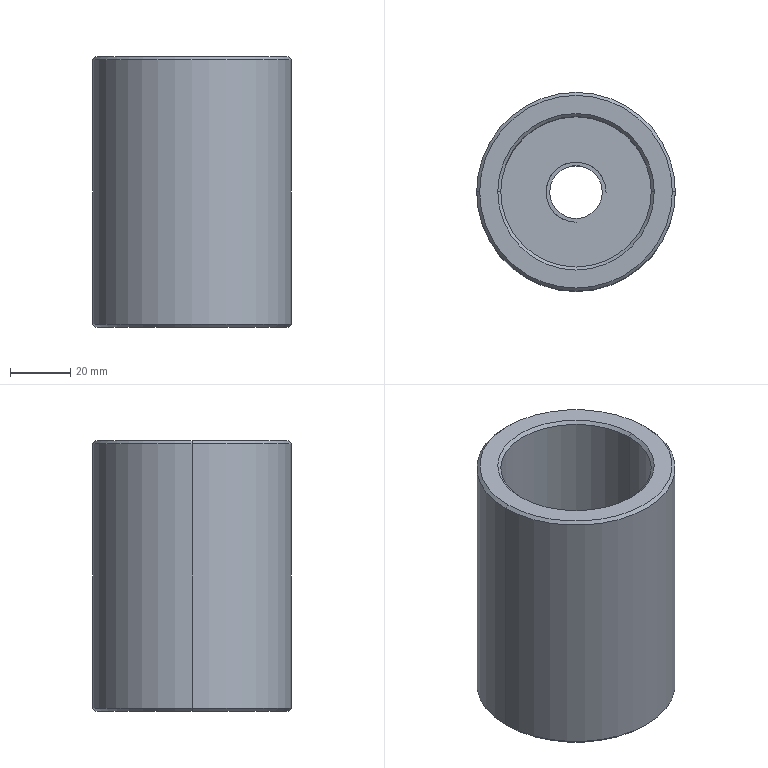Part | Creo | 1 solid | 19 faces | box 66 x 66 x 90 mm | volume 161896 mm3 | cylinder 8 | cone 6 | plane 5 | commonest cylinder face diameters 17.5 x2 50 x2 66 x2 19.94 x1 20 x1
STEP:
#1=CARTESIAN_POINT('',(-258.,289.995,-348.));
#2=VERTEX_POINT('',#1);
#3=CARTESIAN_POINT('',(-208.,289.995,-348.));
#4=VERTEX_POINT('',#3);
#5=CARTESIAN_POINT('',(-233.,289.995,-348.));
#6=DIRECTION('',(0.,0.,1.));
#7=DIRECTION('',(-1.,0.,0.));
#8=AXIS2_PLACEMENT_3D('',#5,#6,#7);
#9=CIRCLE('',#8,25.);
#10=EDGE_CURVE('',#2,#4,#9,.T.);
#11=ORIENTED_EDGE('',*,*,#10,.F.);
#12=CARTESIAN_POINT('',(-233.,289.995,-348.));
#13=DIRECTION('',(0.,0.,1.));
#14=DIRECTION('',(1.,0.,0.));
#15=AXIS2_PLACEMENT_3D('',#12,#13,#14);
#16=CIRCLE('',#15,25.);
#17=EDGE_CURVE('',#4,#2,#16,.T.);
#18=ORIENTED_EDGE('',*,*,#17,.F.);
#19=EDGE_LOOP('',(#11,#18));
#20=FACE_OUTER_BOUND('',#19,.F.);
#21=CARTESIAN_POINT('',(-241.75,289.995,-348.));
#22=VERTEX_POINT('',#21);
#23=CARTESIAN_POINT('',(-224.25,289.995,-348.));
#24=VERTEX_POINT('',#23);
#25=CARTESIAN_POINT('',(-233.,289.995,-348.));
#26=DIRECTION('',(0.,0.,-1.));
#27=DIRECTION('',(-1.,0.,0.));
#28=AXIS2_PLACEMENT_3D('',#25,#26,#27);
#29=CIRCLE('',#28,8.75);
#30=EDGE_CURVE('',#22,#24,#29,.T.);
#31=ORIENTED_EDGE('',*,*,#30,.F.);
#32=CARTESIAN_POINT('',(-233.,289.995,-348.));
#33=DIRECTION('',(0.,0.,-1.));
#34=DIRECTION('',(1.,0.,0.));
#35=AXIS2_PLACEMENT_3D('',#32,#33,#34);
#36=CIRCLE('',#35,8.75);
#37=EDGE_CURVE('',#24,#22,#36,.T.);
#38=ORIENTED_EDGE('',*,*,#37,.F.);
#39=EDGE_LOOP('',(#31,#38));
#40=FACE_BOUND('',#39,.F.);
#41=CARTESIAN_POINT('',(-233.,280.025,-348.));
#42=VERTEX_POINT('',#41);
#43=CARTESIAN_POINT('',(-233.,279.995,-348.));
#44=VERTEX_POINT('',#43);
#45=CARTESIAN_POINT('',(-233.,280.025,-348.));
#46=DIRECTION('',(0.,-1.,0.));
#47=VECTOR('',#46,0.03);
#48=LINE('',#45,#47);
#49=EDGE_CURVE('',#42,#44,#48,.T.);
#50=ORIENTED_EDGE('',*,*,#49,.F.);
#51=CARTESIAN_POINT('',(-223.03,289.995,-348.));
#52=VERTEX_POINT('',#51);
#53=CARTESIAN_POINT('',(-233.,289.995,-348.));
#54=DIRECTION('',(0.,0.,1.));
#55=DIRECTION('',(1.,0.,0.));
#56=AXIS2_PLACEMENT_3D('',#53,#54,#55);
#57=CIRCLE('',#56,9.97);
#58=EDGE_CURVE('',#52,#42,#57,.T.);
#59=ORIENTED_EDGE('',*,*,#58,.F.);
#60=CARTESIAN_POINT('',(-223.,289.995,-348.));
#61=VERTEX_POINT('',#60);
#62=CARTESIAN_POINT('',(-223.,289.995,-348.));
#63=DIRECTION('',(-1.,0.,0.));
#64=VECTOR('',#63,0.03);
#65=LINE('',#62,#64);
#66=EDGE_CURVE('',#61,#52,#65,.T.);
#67=ORIENTED_EDGE('',*,*,#66,.F.);
#68=CARTESIAN_POINT('',(-233.,289.995,-348.));
#69=DIRECTION('',(0.,0.,-1.));
#70=DIRECTION('',(0.,-1.,0.));
#71=AXIS2_PLACEMENT_3D('',#68,#69,#70);
#72=CIRCLE('',#71,10.);
#73=EDGE_CURVE('',#44,#61,#72,.T.);
#74=ORIENTED_EDGE('',*,*,#73,.F.);
#75=EDGE_LOOP('',(#50,#59,#67,#74));
#76=FACE_BOUND('',#75,.F.);
#77=CARTESIAN_POINT('',(-45.,43.995,-348.));
#78=DIRECTION('',(0.,0.,-1.));
#79=DIRECTION('',(0.,1.,0.));
#80=AXIS2_PLACEMENT_3D('',#77,#78,#79);
#81=PLANE('',#80);
#82=ADVANCED_FACE('',(#20,#40,#76),#81,.F.);
#83=ORIENTED_EDGE('',*,*,#49,.T.);
#84=CARTESIAN_POINT('',(-233.,279.995,-366.));
#85=VERTEX_POINT('',#84);
#86=CARTESIAN_POINT('',(-233.,279.995,-348.));
#87=DIRECTION('',(0.,0.,-1.));
#88=VECTOR('',#87,18.);
#89=LINE('',#86,#88);
#90=EDGE_CURVE('',#44,#85,#89,.T.);
#91=ORIENTED_EDGE('',*,*,#90,.T.);
#92=CARTESIAN_POINT('',(-233.,280.025,-366.));
#93=VERTEX_POINT('',#92);
#94=CARTESIAN_POINT('',(-233.,279.995,-366.));
#95=DIRECTION('',(0.,1.,0.));
#96=VECTOR('',#95,0.03);
#97=LINE('',#94,#96);
#98=EDGE_CURVE('',#85,#93,#97,.T.);
#99=ORIENTED_EDGE('',*,*,#98,.T.);
#100=CARTESIAN_POINT('',(-233.,280.025,-366.));
#101=DIRECTION('',(0.,0.,1.));
#102=VECTOR('',#101,18.);
#103=LINE('',#100,#102);
#104=EDGE_CURVE('',#93,#42,#103,.T.);
#105=ORIENTED_EDGE('',*,*,#104,.T.);
#106=EDGE_LOOP('',(#83,#91,#99,#105));
#107=FACE_OUTER_BOUND('',#106,.F.);
#108=CARTESIAN_POINT('',(-233.,284.995,-321.));
#109=DIRECTION('',(-1.,0.,0.));
#110=DIRECTION('',(0.,0.,-1.));
#111=AXIS2_PLACEMENT_3D('',#108,#109,#110);
#112=PLANE('',#111);
#113=ADVANCED_FACE('',(#107),#112,.T.);
#114=ORIENTED_EDGE('',*,*,#90,.F.);
#115=ORIENTED_EDGE('',*,*,#73,.T.);
#116=CARTESIAN_POINT('',(-223.,289.995,-366.));
#117=VERTEX_POINT('',#116);
#118=CARTESIAN_POINT('',(-223.,289.995,-366.));
#119=DIRECTION('',(0.,0.,1.));
#120=VECTOR('',#119,18.);
#121=LINE('',#118,#120);
#122=EDGE_CURVE('',#117,#61,#121,.T.);
#123=ORIENTED_EDGE('',*,*,#122,.F.);
#124=CARTESIAN_POINT('',(-243.,289.995,-366.));
#125=VERTEX_POINT('',#124);
#126=CARTESIAN_POINT('',(-233.,289.995,-366.));
#127=DIRECTION('',(0.,0.,1.));
#128=DIRECTION('',(1.,0.,0.));
#129=AXIS2_PLACEMENT_3D('',#126,#127,#128);
#130=CIRCLE('',#129,10.);
#131=EDGE_CURVE('',#117,#125,#130,.T.);
#132=ORIENTED_EDGE('',*,*,#131,.T.);
#133=CARTESIAN_POINT('',(-233.,289.995,-366.));
#134=DIRECTION('',(0.,0.,1.));
#135=DIRECTION('',(-1.,0.,0.));
#136=AXIS2_PLACEMENT_3D('',#133,#134,#135);
#137=CIRCLE('',#136,10.);
#138=EDGE_CURVE('',#125,#85,#137,.T.);
#139=ORIENTED_EDGE('',*,*,#138,.T.);
#140=EDGE_LOOP('',(#114,#115,#123,#132,#139));
#141=FACE_OUTER_BOUND('',#140,.F.);
#142=CARTESIAN_POINT('',(-233.,289.995,-366.));
#143=DIRECTION('',(0.,0.,1.));
#144=DIRECTION('',(1.,0.,0.));
#145=AXIS2_PLACEMENT_3D('',#142,#143,#144);
#146=CYLINDRICAL_SURFACE('',#145,10.);
#147=ADVANCED_FACE('',(#141),#146,.F.);
#148=ORIENTED_EDGE('',*,*,#66,.T.);
#149=CARTESIAN_POINT('',(-223.03,289.995,-366.));
#150=VERTEX_POINT('',#149);
#151=CARTESIAN_POINT('',(-223.03,289.995,-348.));
#152=DIRECTION('',(0.,0.,-1.));
#153=VECTOR('',#152,18.);
#154=LINE('',#151,#153);
#155=EDGE_CURVE('',#52,#150,#154,.T.);
#156=ORIENTED_EDGE('',*,*,#155,.T.);
#157=CARTESIAN_POINT('',(-223.03,289.995,-366.));
#158=DIRECTION('',(1.,0.,0.));
#159=VECTOR('',#158,0.03);
#160=LINE('',#157,#159);
#161=EDGE_CURVE('',#150,#117,#160,.T.);
#162=ORIENTED_EDGE('',*,*,#161,.T.);
#163=ORIENTED_EDGE('',*,*,#122,.T.);
#164=EDGE_LOOP('',(#148,#156,#162,#163));
#165=FACE_OUTER_BOUND('',#164,.F.);
#166=CARTESIAN_POINT('',(-228.,289.995,-321.));
#167=DIRECTION('',(0.,1.,0.));
#168=DIRECTION('',(0.,0.,1.));
#169=AXIS2_PLACEMENT_3D('',#166,#167,#168);
#170=PLANE('',#169);
#171=ADVANCED_FACE('',(#165),#170,.T.);
#172=ORIENTED_EDGE('',*,*,#58,.T.);
#173=ORIENTED_EDGE('',*,*,#104,.F.);
#174=CARTESIAN_POINT('',(-242.97,289.995,-366.));
#175=VERTEX_POINT('',#174);
#176=CARTESIAN_POINT('',(-233.,289.995,-366.));
#177=DIRECTION('',(0.,0.,-1.));
#178=DIRECTION('',(0.,-1.,0.));
#179=AXIS2_PLACEMENT_3D('',#176,#177,#178);
#180=CIRCLE('',#179,9.97);
#181=EDGE_CURVE('',#93,#175,#180,.T.);
#182=ORIENTED_EDGE('',*,*,#181,.T.);
#183=CARTESIAN_POINT('',(-233.,289.995,-366.));
#184=DIRECTION('',(0.,0.,-1.));
#185=DIRECTION('',(-1.,0.,0.));
#186=AXIS2_PLACEMENT_3D('',#183,#184,#185);
#187=CIRCLE('',#186,9.97);
#188=EDGE_CURVE('',#175,#150,#187,.T.);
#189=ORIENTED_EDGE('',*,*,#188,.T.);
#190=ORIENTED_EDGE('',*,*,#155,.F.);
#191=EDGE_LOOP('',(#172,#173,#182,#189,#190));
#192=FACE_OUTER_BOUND('',#191,.F.);
#193=CARTESIAN_POINT('',(-233.,289.995,-366.));
#194=DIRECTION('',(0.,0.,1.));
#195=DIRECTION('',(1.,0.,0.));
#196=AXIS2_PLACEMENT_3D('',#193,#194,#195);
#197=CYLINDRICAL_SURFACE('',#196,9.97);
#198=ADVANCED_FACE('',(#192),#197,.T.);
#199=CARTESIAN_POINT('',(-201.,289.995,-366.));
#200=VERTEX_POINT('',#199);
#201=CARTESIAN_POINT('',(-265.,289.995,-366.));
#202=VERTEX_POINT('',#201);
#203=CARTESIAN_POINT('',(-233.,289.995,-366.));
#204=DIRECTION('',(0.,0.,-1.));
#205=DIRECTION('',(1.,0.,0.));
#206=AXIS2_PLACEMENT_3D('',#203,#204,#205);
#207=CIRCLE('',#206,32.);
#208=EDGE_CURVE('',#200,#202,#207,.T.);
#209=ORIENTED_EDGE('',*,*,#208,.F.);
#210=CARTESIAN_POINT('',(-233.,289.995,-366.));
#211=DIRECTION('',(0.,0.,-1.));
#212=DIRECTION('',(-1.,0.,0.));
#213=AXIS2_PLACEMENT_3D('',#210,#211,#212);
#214=CIRCLE('',#213,32.);
#215=EDGE_CURVE('',#202,#200,#214,.T.);
#216=ORIENTED_EDGE('',*,*,#215,.F.);
#217=EDGE_LOOP('',(#209,#216));
#218=FACE_OUTER_BOUND('',#217,.F.);
#219=ORIENTED_EDGE('',*,*,#161,.F.);
#220=ORIENTED_EDGE('',*,*,#188,.F.);
#221=ORIENTED_EDGE('',*,*,#181,.F.);
#222=ORIENTED_EDGE('',*,*,#98,.F.);
#223=ORIENTED_EDGE('',*,*,#138,.F.);
#224=ORIENTED_EDGE('',*,*,#131,.F.);
#225=EDGE_LOOP('',(#219,#220,#221,#222,#223,#224));
#226=FACE_BOUND('',#225,.F.);
#227=CARTESIAN_POINT('',(-224.25,289.995,-366.));
#228=VERTEX_POINT('',#227);
#229=CARTESIAN_POINT('',(-241.75,289.995,-366.));
#230=VERTEX_POINT('',#229);
#231=CARTESIAN_POINT('',(-233.,289.995,-366.));
#232=DIRECTION('',(0.,0.,1.));
#233=DIRECTION('',(1.,0.,0.));
#234=AXIS2_PLACEMENT_3D('',#231,#232,#233);
#235=CIRCLE('',#234,8.75);
#236=EDGE_CURVE('',#228,#230,#235,.T.);
#237=ORIENTED_EDGE('',*,*,#236,.F.);
#238=CARTESIAN_POINT('',(-233.,289.995,-366.));
#239=DIRECTION('',(0.,0.,1.));
#240=DIRECTION('',(-1.,0.,0.));
#241=AXIS2_PLACEMENT_3D('',#238,#239,#240);
#242=CIRCLE('',#241,8.75);
#243=EDGE_CURVE('',#230,#228,#242,.T.);
#244=ORIENTED_EDGE('',*,*,#243,.F.);
#245=EDGE_LOOP('',(#237,#244));
#246=FACE_BOUND('',#245,.F.);
#247=CARTESIAN_POINT('',(-45.,43.995,-366.));
#248=DIRECTION('',(0.,0.,-1.));
#249=DIRECTION('',(1.,0.,0.));
#250=AXIS2_PLACEMENT_3D('',#247,#248,#249);
#251=PLANE('',#250);
#252=ADVANCED_FACE('',(#218,#226,#246),#251,.T.);
#253=ORIENTED_EDGE('',*,*,#208,.T.);
#254=CARTESIAN_POINT('',(-266.,289.995,-365.));
#255=VERTEX_POINT('',#254);
#256=CARTESIAN_POINT('',(-265.,289.995,-366.));
#257=DIRECTION('',(-0.7071,0.,0.7071));
#258=VECTOR('',#257,1.414);
#259=LINE('',#256,#258);
#260=EDGE_CURVE('',#202,#255,#259,.T.);
#261=ORIENTED_EDGE('',*,*,#260,.T.);
#262=CARTESIAN_POINT('',(-200.,289.995,-365.));
#263=VERTEX_POINT('',#262);
#264=CARTESIAN_POINT('',(-233.,289.995,-365.));
#265=DIRECTION('',(0.,0.,-1.));
#266=DIRECTION('',(1.,0.,0.));
#267=AXIS2_PLACEMENT_3D('',#264,#265,#266);
#268=CIRCLE('',#267,33.);
#269=EDGE_CURVE('',#263,#255,#268,.T.);
#270=ORIENTED_EDGE('',*,*,#269,.F.);
#271=CARTESIAN_POINT('',(-201.,289.995,-366.));
#272=DIRECTION('',(0.7071,0.,0.7071));
#273=VECTOR('',#272,1.414);
#274=LINE('',#271,#273);
#275=EDGE_CURVE('',#200,#263,#274,.T.);
#276=ORIENTED_EDGE('',*,*,#275,.F.);
#277=EDGE_LOOP('',(#253,#261,#270,#276));
#278=FACE_OUTER_BOUND('',#277,.F.);
#279=CARTESIAN_POINT('',(-233.,289.995,-365.5));
#280=DIRECTION('',(0.,0.,1.));
#281=DIRECTION('',(-1.,0.,0.));
#282=AXIS2_PLACEMENT_3D('',#279,#280,#281);
#283=CONICAL_SURFACE('',#282,32.5,45.);
#284=ADVANCED_FACE('',(#278),#283,.T.);
#285=ORIENTED_EDGE('',*,*,#215,.T.);
#286=ORIENTED_EDGE('',*,*,#275,.T.);
#287=CARTESIAN_POINT('',(-233.,289.995,-365.));
#288=DIRECTION('',(0.,0.,-1.));
#289=DIRECTION('',(-1.,0.,0.));
#290=AXIS2_PLACEMENT_3D('',#287,#288,#289);
#291=CIRCLE('',#290,33.);
#292=EDGE_CURVE('',#255,#263,#291,.T.);
#293=ORIENTED_EDGE('',*,*,#292,.F.);
#294=ORIENTED_EDGE('',*,*,#260,.F.);
#295=EDGE_LOOP('',(#285,#286,#293,#294));
#296=FACE_OUTER_BOUND('',#295,.F.);
#297=CARTESIAN_POINT('',(-233.,289.995,-365.5));
#298=DIRECTION('',(0.,0.,1.));
#299=DIRECTION('',(-1.,0.,0.));
#300=AXIS2_PLACEMENT_3D('',#297,#298,#299);
#301=CONICAL_SURFACE('',#300,32.5,45.);
#302=ADVANCED_FACE('',(#296),#301,.T.);
#303=ORIENTED_EDGE('',*,*,#292,.T.);
#304=CARTESIAN_POINT('',(-200.,289.995,-277.));
#305=VERTEX_POINT('',#304);
#306=CARTESIAN_POINT('',(-200.,289.995,-277.));
#307=DIRECTION('',(0.,0.,-1.));
#308=VECTOR('',#307,88.);
#309=LINE('',#306,#308);
#310=EDGE_CURVE('',#305,#263,#309,.T.);
#311=ORIENTED_EDGE('',*,*,#310,.F.);
#312=CARTESIAN_POINT('',(-266.,289.995,-277.));
#313=VERTEX_POINT('',#312);
#314=CARTESIAN_POINT('',(-233.,289.995,-277.));
#315=DIRECTION('',(0.,0.,1.));
#316=DIRECTION('',(1.,0.,0.));
#317=AXIS2_PLACEMENT_3D('',#314,#315,#316);
#318=CIRCLE('',#317,33.);
#319=EDGE_CURVE('',#305,#313,#318,.T.);
#320=ORIENTED_EDGE('',*,*,#319,.T.);
#321=CARTESIAN_POINT('',(-266.,289.995,-277.));
#322=DIRECTION('',(0.,0.,-1.));
#323=VECTOR('',#322,88.);
#324=LINE('',#321,#323);
#325=EDGE_CURVE('',#313,#255,#324,.T.);
#326=ORIENTED_EDGE('',*,*,#325,.T.);
#327=EDGE_LOOP('',(#303,#311,#320,#326));
#328=FACE_OUTER_BOUND('',#327,.F.);
#329=CARTESIAN_POINT('',(-233.,289.995,-396.));
#330=DIRECTION('',(0.,0.,-1.));
#331=DIRECTION('',(1.,0.,0.));
#332=AXIS2_PLACEMENT_3D('',#329,#330,#331);
#333=CYLINDRICAL_SURFACE('',#332,33.);
#334=ADVANCED_FACE('',(#328),#333,.T.);
#335=ORIENTED_EDGE('',*,*,#269,.T.);
#336=ORIENTED_EDGE('',*,*,#325,.F.);
#337=CARTESIAN_POINT('',(-233.,289.995,-277.));
#338=DIRECTION('',(0.,0.,1.));
#339=DIRECTION('',(-1.,0.,0.));
#340=AXIS2_PLACEMENT_3D('',#337,#338,#339);
#341=CIRCLE('',#340,33.);
#342=EDGE_CURVE('',#313,#305,#341,.T.);
#343=ORIENTED_EDGE('',*,*,#342,.T.);
#344=ORIENTED_EDGE('',*,*,#310,.T.);
#345=EDGE_LOOP('',(#335,#336,#343,#344));
#346=FACE_OUTER_BOUND('',#345,.F.);
#347=CARTESIAN_POINT('',(-233.,289.995,-396.));
#348=DIRECTION('',(0.,0.,-1.));
#349=DIRECTION('',(1.,0.,0.));
#350=AXIS2_PLACEMENT_3D('',#347,#348,#349);
#351=CYLINDRICAL_SURFACE('',#350,33.);
#352=ADVANCED_FACE('',(#346),#351,.T.);
#353=CARTESIAN_POINT('',(-265.,289.995,-276.));
#354=VERTEX_POINT('',#353);
#355=CARTESIAN_POINT('',(-201.,289.995,-276.));
#356=VERTEX_POINT('',#355);
#357=CARTESIAN_POINT('',(-233.,289.995,-276.));
#358=DIRECTION('',(0.,0.,1.));
#359=DIRECTION('',(-1.,0.,0.));
#360=AXIS2_PLACEMENT_3D('',#357,#358,#359);
#361=CIRCLE('',#360,32.);
#362=EDGE_CURVE('',#354,#356,#361,.T.);
#363=ORIENTED_EDGE('',*,*,#362,.T.);
#364=CARTESIAN_POINT('',(-201.,289.995,-276.));
#365=DIRECTION('',(0.7071,0.,-0.7071));
#366=VECTOR('',#365,1.414);
#367=LINE('',#364,#366);
#368=EDGE_CURVE('',#356,#305,#367,.T.);
#369=ORIENTED_EDGE('',*,*,#368,.T.);
#370=ORIENTED_EDGE('',*,*,#342,.F.);
#371=CARTESIAN_POINT('',(-265.,289.995,-276.));
#372=DIRECTION('',(-0.7071,0.,-0.7071));
#373=VECTOR('',#372,1.414);
#374=LINE('',#371,#373);
#375=EDGE_CURVE('',#354,#313,#374,.T.);
#376=ORIENTED_EDGE('',*,*,#375,.F.);
#377=EDGE_LOOP('',(#363,#369,#370,#376));
#378=FACE_OUTER_BOUND('',#377,.F.);
#379=CARTESIAN_POINT('',(-233.,289.995,-276.5));
#380=DIRECTION('',(0.,0.,-1.));
#381=DIRECTION('',(-1.,0.,0.));
#382=AXIS2_PLACEMENT_3D('',#379,#380,#381);
#383=CONICAL_SURFACE('',#382,32.5,45.);
#384=ADVANCED_FACE('',(#378),#383,.T.);
#385=ORIENTED_EDGE('',*,*,#362,.F.);
#386=CARTESIAN_POINT('',(-233.,289.995,-276.));
#387=DIRECTION('',(0.,0.,1.));
#388=DIRECTION('',(1.,0.,0.));
#389=AXIS2_PLACEMENT_3D('',#386,#387,#388);
#390=CIRCLE('',#389,32.);
#391=EDGE_CURVE('',#356,#354,#390,.T.);
#392=ORIENTED_EDGE('',*,*,#391,.F.);
#393=EDGE_LOOP('',(#385,#392));
#394=FACE_OUTER_BOUND('',#393,.F.);
#395=CARTESIAN_POINT('',(-259.,289.995,-276.));
#396=VERTEX_POINT('',#395);
#397=CARTESIAN_POINT('',(-207.,289.995,-276.));
#398=VERTEX_POINT('',#397);
#399=CARTESIAN_POINT('',(-233.,289.995,-276.));
#400=DIRECTION('',(0.,0.,-1.));
#401=DIRECTION('',(-1.,0.,0.));
#402=AXIS2_PLACEMENT_3D('',#399,#400,#401);
#403=CIRCLE('',#402,26.);
#404=EDGE_CURVE('',#396,#398,#403,.T.);
#405=ORIENTED_EDGE('',*,*,#404,.F.);
#406=CARTESIAN_POINT('',(-233.,289.995,-276.));
#407=DIRECTION('',(0.,0.,-1.));
#408=DIRECTION('',(1.,0.,0.));
#409=AXIS2_PLACEMENT_3D('',#406,#407,#408);
#410=CIRCLE('',#409,26.);
#411=EDGE_CURVE('',#398,#396,#410,.T.);
#412=ORIENTED_EDGE('',*,*,#411,.F.);
#413=EDGE_LOOP('',(#405,#412));
#414=FACE_BOUND('',#413,.F.);
#415=CARTESIAN_POINT('',(-45.,43.995,-276.));
#416=DIRECTION('',(0.,0.,-1.));
#417=DIRECTION('',(1.,0.,0.));
#418=AXIS2_PLACEMENT_3D('',#415,#416,#417);
#419=PLANE('',#418);
#420=ADVANCED_FACE('',(#394,#414),#419,.F.);
#421=ORIENTED_EDGE('',*,*,#404,.T.);
#422=CARTESIAN_POINT('',(-208.,289.995,-277.));
#423=VERTEX_POINT('',#422);
#424=CARTESIAN_POINT('',(-208.,289.995,-277.));
#425=DIRECTION('',(0.7071,0.,0.7071));
#426=VECTOR('',#425,1.414);
#427=LINE('',#424,#426);
#428=EDGE_CURVE('',#423,#398,#427,.T.);
#429=ORIENTED_EDGE('',*,*,#428,.F.);
#430=CARTESIAN_POINT('',(-258.,289.995,-277.));
#431=VERTEX_POINT('',#430);
#432=CARTESIAN_POINT('',(-233.,289.995,-277.));
#433=DIRECTION('',(0.,0.,-1.));
#434=DIRECTION('',(-1.,0.,0.));
#435=AXIS2_PLACEMENT_3D('',#432,#433,#434);
#436=CIRCLE('',#435,25.);
#437=EDGE_CURVE('',#431,#423,#436,.T.);
#438=ORIENTED_EDGE('',*,*,#437,.F.);
#439=CARTESIAN_POINT('',(-258.,289.995,-277.));
#440=DIRECTION('',(-0.7071,0.,0.7071));
#441=VECTOR('',#440,1.414);
#442=LINE('',#439,#441);
#443=EDGE_CURVE('',#431,#396,#442,.T.);
#444=ORIENTED_EDGE('',*,*,#443,.T.);
#445=EDGE_LOOP('',(#421,#429,#438,#444));
#446=FACE_OUTER_BOUND('',#445,.F.);
#447=CARTESIAN_POINT('',(-233.,289.995,-276.5));
#448=DIRECTION('',(0.,0.,1.));
#449=DIRECTION('',(-1.,0.,0.));
#450=AXIS2_PLACEMENT_3D('',#447,#448,#449);
#451=CONICAL_SURFACE('',#450,25.5,45.);
#452=ADVANCED_FACE('',(#446),#451,.F.);
#453=ORIENTED_EDGE('',*,*,#411,.T.);
#454=ORIENTED_EDGE('',*,*,#443,.F.);
#455=CARTESIAN_POINT('',(-233.,289.995,-277.));
#456=DIRECTION('',(0.,0.,-1.));
#457=DIRECTION('',(1.,0.,0.));
#458=AXIS2_PLACEMENT_3D('',#455,#456,#457);
#459=CIRCLE('',#458,25.);
#460=EDGE_CURVE('',#423,#431,#459,.T.);
#461=ORIENTED_EDGE('',*,*,#460,.F.);
#462=ORIENTED_EDGE('',*,*,#428,.T.);
#463=EDGE_LOOP('',(#453,#454,#461,#462));
#464=FACE_OUTER_BOUND('',#463,.F.);
#465=CARTESIAN_POINT('',(-233.,289.995,-276.5));
#466=DIRECTION('',(0.,0.,1.));
#467=DIRECTION('',(-1.,0.,0.));
#468=AXIS2_PLACEMENT_3D('',#465,#466,#467);
#469=CONICAL_SURFACE('',#468,25.5,45.);
#470=ADVANCED_FACE('',(#464),#469,.F.);
#471=ORIENTED_EDGE('',*,*,#10,.T.);
#472=CARTESIAN_POINT('',(-208.,289.995,-277.));
#473=DIRECTION('',(0.,0.,-1.));
#474=VECTOR('',#473,71.);
#475=LINE('',#472,#474);
#476=EDGE_CURVE('',#423,#4,#475,.T.);
#477=ORIENTED_EDGE('',*,*,#476,.F.);
#478=ORIENTED_EDGE('',*,*,#460,.T.);
#479=CARTESIAN_POINT('',(-258.,289.995,-277.));
#480=DIRECTION('',(0.,0.,-1.));
#481=VECTOR('',#480,71.);
#482=LINE('',#479,#481);
#483=EDGE_CURVE('',#431,#2,#482,.T.);
#484=ORIENTED_EDGE('',*,*,#483,.T.);
#485=EDGE_LOOP('',(#471,#477,#478,#484));
#486=FACE_OUTER_BOUND('',#485,.F.);
#487=CARTESIAN_POINT('',(-233.,289.995,-396.));
#488=DIRECTION('',(0.,0.,-1.));
#489=DIRECTION('',(1.,0.,0.));
#490=AXIS2_PLACEMENT_3D('',#487,#488,#489);
#491=CYLINDRICAL_SURFACE('',#490,25.);
#492=ADVANCED_FACE('',(#486),#491,.F.);
#493=ORIENTED_EDGE('',*,*,#17,.T.);
#494=ORIENTED_EDGE('',*,*,#483,.F.);
#495=ORIENTED_EDGE('',*,*,#437,.T.);
#496=ORIENTED_EDGE('',*,*,#476,.T.);
#497=EDGE_LOOP('',(#493,#494,#495,#496));
#498=FACE_OUTER_BOUND('',#497,.F.);
#499=CARTESIAN_POINT('',(-233.,289.995,-396.));
#500=DIRECTION('',(0.,0.,-1.));
#501=DIRECTION('',(1.,0.,0.));
#502=AXIS2_PLACEMENT_3D('',#499,#500,#501);
#503=CYLINDRICAL_SURFACE('',#502,25.);
#504=ADVANCED_FACE('',(#498),#503,.F.);
#505=ORIENTED_EDGE('',*,*,#391,.T.);
#506=ORIENTED_EDGE('',*,*,#375,.T.);
#507=ORIENTED_EDGE('',*,*,#319,.F.);
#508=ORIENTED_EDGE('',*,*,#368,.F.);
#509=EDGE_LOOP('',(#505,#506,#507,#508));
#510=FACE_OUTER_BOUND('',#509,.F.);
#511=CARTESIAN_POINT('',(-233.,289.995,-276.5));
#512=DIRECTION('',(0.,0.,-1.));
#513=DIRECTION('',(-1.,0.,0.));
#514=AXIS2_PLACEMENT_3D('',#511,#512,#513);
#515=CONICAL_SURFACE('',#514,32.5,45.);
#516=ADVANCED_FACE('',(#510),#515,.T.);
#517=ORIENTED_EDGE('',*,*,#236,.T.);
#518=CARTESIAN_POINT('',(-241.75,289.995,-366.));
#519=DIRECTION('',(0.,0.,1.));
#520=VECTOR('',#519,18.);
#521=LINE('',#518,#520);
#522=EDGE_CURVE('',#230,#22,#521,.T.);
#523=ORIENTED_EDGE('',*,*,#522,.T.);
#524=ORIENTED_EDGE('',*,*,#30,.T.);
#525=CARTESIAN_POINT('',(-224.25,289.995,-366.));
#526=DIRECTION('',(0.,0.,1.));
#527=VECTOR('',#526,18.);
#528=LINE('',#525,#527);
#529=EDGE_CURVE('',#228,#24,#528,.T.);
#530=ORIENTED_EDGE('',*,*,#529,.F.);
#531=EDGE_LOOP('',(#517,#523,#524,#530));
#532=FACE_OUTER_BOUND('',#531,.F.);
#533=CARTESIAN_POINT('',(-233.,289.995,-366.));
#534=DIRECTION('',(0.,0.,1.));
#535=DIRECTION('',(1.,0.,0.));
#536=AXIS2_PLACEMENT_3D('',#533,#534,#535);
#537=CYLINDRICAL_SURFACE('',#536,8.75);
#538=ADVANCED_FACE('',(#532),#537,.F.);
#539=ORIENTED_EDGE('',*,*,#243,.T.);
#540=ORIENTED_EDGE('',*,*,#529,.T.);
#541=ORIENTED_EDGE('',*,*,#37,.T.);
#542=ORIENTED_EDGE('',*,*,#522,.F.);
#543=EDGE_LOOP('',(#539,#540,#541,#542));
#544=FACE_OUTER_BOUND('',#543,.F.);
#545=CARTESIAN_POINT('',(-233.,289.995,-366.));
#546=DIRECTION('',(0.,0.,1.));
#547=DIRECTION('',(1.,0.,0.));
#548=AXIS2_PLACEMENT_3D('',#545,#546,#547);
#549=CYLINDRICAL_SURFACE('',#548,8.75);
#550=ADVANCED_FACE('',(#544),#549,.F.);
#551=CLOSED_SHELL('',(#82,#113,#147,#171,#198,#252,#284,#302,#334,#352,#384,#420,#452,#470,#492,#504,#516,#538,#550));
#552=MANIFOLD_SOLID_BREP('',#551);
#553=(LENGTH_UNIT()NAMED_UNIT(*)SI_UNIT(.MILLI.,.METRE.));
#554=UNCERTAINTY_MEASURE_WITH_UNIT(LENGTH_MEASURE(0.01297),#553,'','');
#555=(NAMED_UNIT(*)PLANE_ANGLE_UNIT()SI_UNIT($,.RADIAN.));
#556=PLANE_ANGLE_MEASURE_WITH_UNIT(PLANE_ANGLE_MEASURE(0.01745),#555);
#557=(CONVERSION_BASED_UNIT('DEGREE',#556)NAMED_UNIT(*)PLANE_ANGLE_UNIT());
#558=(NAMED_UNIT(*)SI_UNIT($,.STERADIAN.)SOLID_ANGLE_UNIT());
#559=(GEOMETRIC_REPRESENTATION_CONTEXT(3)GLOBAL_UNCERTAINTY_ASSIGNED_CONTEXT((#554))GLOBAL_UNIT_ASSIGNED_CONTEXT((#553,#557,#558))REPRESENTATION_CONTEXT('',''));
#560=ADVANCED_BREP_SHAPE_REPRESENTATION('',(#552),#559);